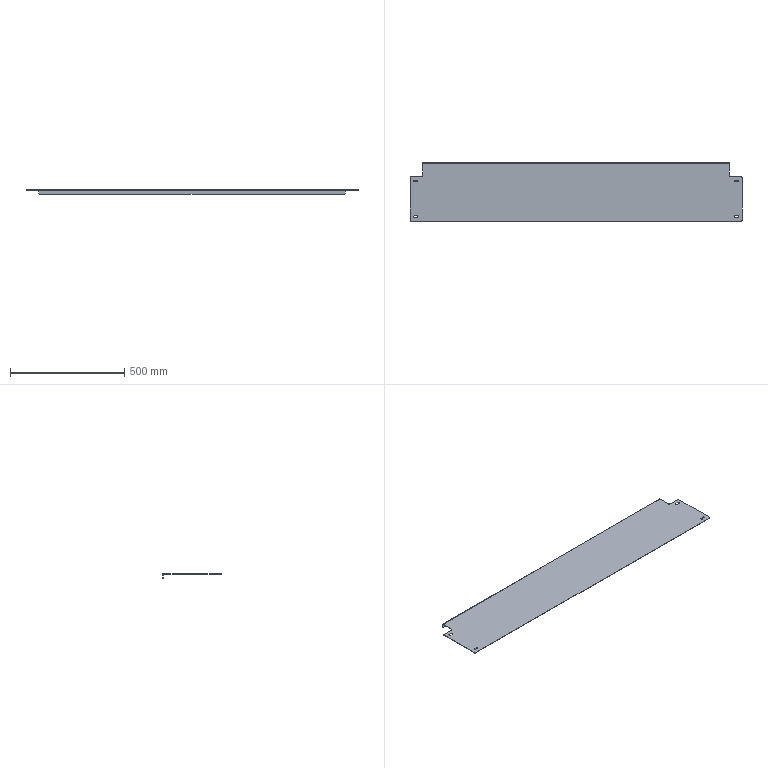Part | STEP file | DCV-000-011 | 1 solid | 50 faces | box 1450 x 256 x 20 mm | volume 581295 mm3 | cylinder 26 | plane 24 | commonest cylinder face diameters 10 x16 8 x6 9 x2 3 x1 6 x1